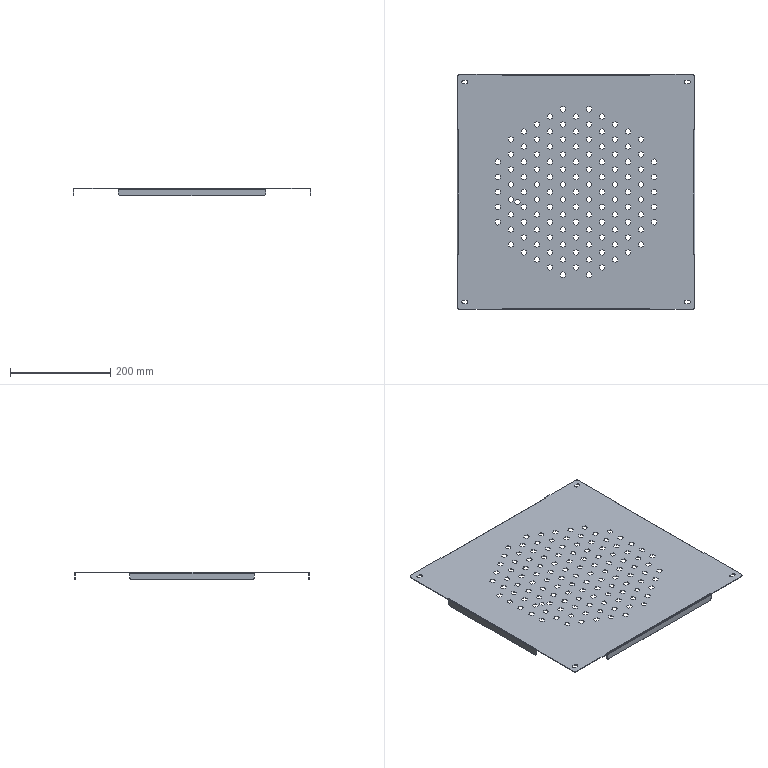Part | SolidWorks | features BaseBody 1 | 1 solid | 834 faces | box 473 x 468 x 15 mm | volume 269570 mm3 | plane 802 | cylinder 32 | commonest cylinder face diameters 7 x12 10 x12 2 x4 4.4 x4